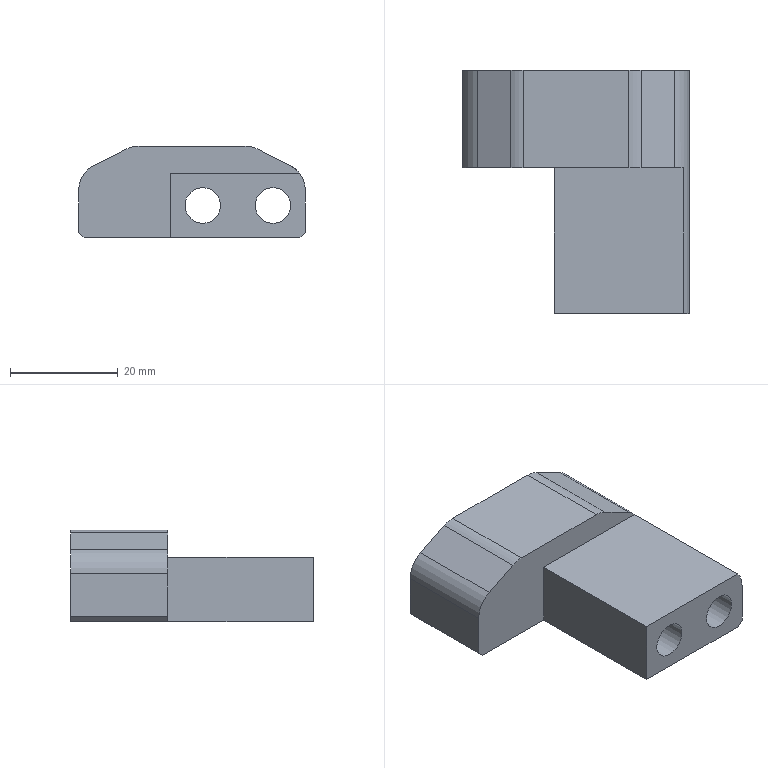Part | STEP file | solid 59 | 1 solid | 19 faces | box 42 x 45 x 17 mm | volume 16851 mm3 | plane 13 | cylinder 6 | commonest cylinder face diameters 10 x4 6.6 x2